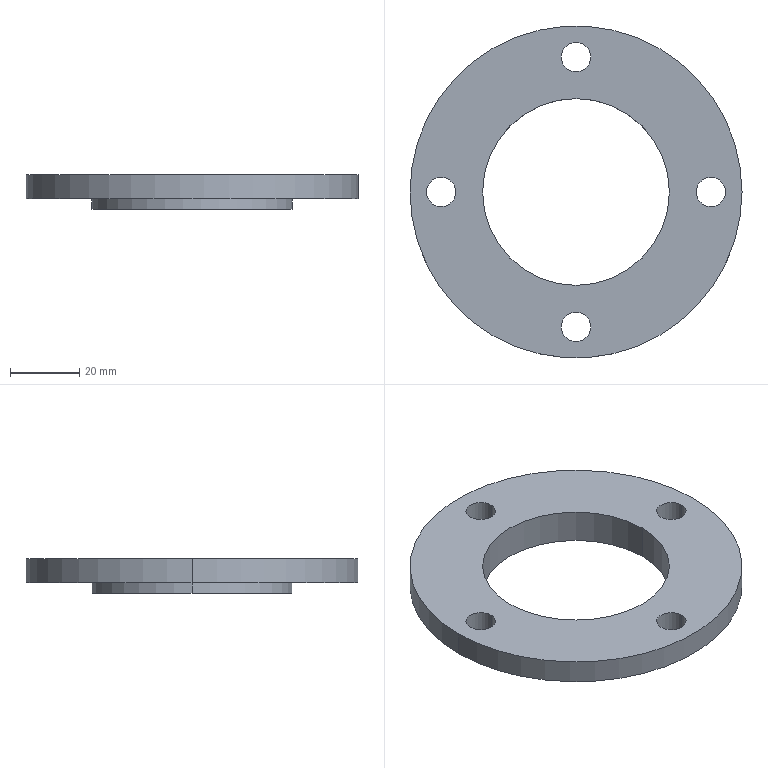Part | SolidWorks | features BaseBody 1 | 1 solid | 17 faces | box 96 x 96 x 10 mm | volume 34103 mm3 | cylinder 14 | plane 3 | commonest cylinder face diameters 8.5 x8 54 x2 58 x2 96 x2
STEP:
#1=CARTESIAN_POINT('',(29.,0.,-7.));
#2=VERTEX_POINT('',#1);
#3=CARTESIAN_POINT('',(29.,0.,-10.));
#4=VERTEX_POINT('',#3);
#5=CARTESIAN_POINT('',(29.,0.,-7.));
#6=DIRECTION('',(0.,0.,-1.));
#7=VECTOR('',#6,1000.);
#8=LINE('',#5,#7);
#9=EDGE_CURVE('',#2,#4,#8,.T.);
#10=ORIENTED_EDGE('',*,*,#9,.F.);
#11=CARTESIAN_POINT('',(-29.,0.,-7.));
#12=VERTEX_POINT('',#11);
#13=CARTESIAN_POINT('',(0.,0.,-7.));
#14=DIRECTION('',(0.,0.,-1.));
#15=DIRECTION('',(-1.,0.,0.));
#16=AXIS2_PLACEMENT_3D('',#13,#14,#15);
#17=CIRCLE('',#16,29.);
#18=EDGE_CURVE('',#2,#12,#17,.T.);
#19=ORIENTED_EDGE('',*,*,#18,.T.);
#20=CARTESIAN_POINT('',(-29.,0.,-10.));
#21=VERTEX_POINT('',#20);
#22=CARTESIAN_POINT('',(-29.,0.,-7.));
#23=DIRECTION('',(0.,0.,-1.));
#24=VECTOR('',#23,1000.);
#25=LINE('',#22,#24);
#26=EDGE_CURVE('',#12,#21,#25,.T.);
#27=ORIENTED_EDGE('',*,*,#26,.T.);
#28=CARTESIAN_POINT('',(0.,0.,-10.));
#29=DIRECTION('',(0.,0.,-1.));
#30=DIRECTION('',(-1.,0.,0.));
#31=AXIS2_PLACEMENT_3D('',#28,#29,#30);
#32=CIRCLE('',#31,29.);
#33=EDGE_CURVE('',#4,#21,#32,.T.);
#34=ORIENTED_EDGE('',*,*,#33,.F.);
#35=EDGE_LOOP('',(#10,#19,#27,#34));
#36=FACE_OUTER_BOUND('',#35,.T.);
#37=CARTESIAN_POINT('',(0.,0.,-7.));
#38=DIRECTION('',(0.,0.,-1.));
#39=DIRECTION('',(-1.,0.,0.));
#40=AXIS2_PLACEMENT_3D('',#37,#38,#39);
#41=CYLINDRICAL_SURFACE('',#40,29.);
#42=ADVANCED_FACE('',(#36),#41,.T.);
#43=CARTESIAN_POINT('',(4.25,39.,-7.));
#44=VERTEX_POINT('',#43);
#45=CARTESIAN_POINT('',(-4.25,39.,-7.));
#46=VERTEX_POINT('',#45);
#47=CARTESIAN_POINT('',(0.,39.,-7.));
#48=DIRECTION('',(0.,0.,1.));
#49=DIRECTION('',(-1.,0.,0.));
#50=AXIS2_PLACEMENT_3D('',#47,#48,#49);
#51=CIRCLE('',#50,4.25);
#52=EDGE_CURVE('',#44,#46,#51,.T.);
#53=ORIENTED_EDGE('',*,*,#52,.T.);
#54=CARTESIAN_POINT('',(0.,39.,-7.));
#55=DIRECTION('',(0.,0.,1.));
#56=DIRECTION('',(-1.,0.,0.));
#57=AXIS2_PLACEMENT_3D('',#54,#55,#56);
#58=CIRCLE('',#57,4.25);
#59=EDGE_CURVE('',#46,#44,#58,.T.);
#60=ORIENTED_EDGE('',*,*,#59,.T.);
#61=EDGE_LOOP('',(#53,#60));
#62=FACE_BOUND('',#61,.T.);
#63=CARTESIAN_POINT('',(43.25,0.,-7.));
#64=VERTEX_POINT('',#63);
#65=CARTESIAN_POINT('',(34.75,0.,-7.));
#66=VERTEX_POINT('',#65);
#67=CARTESIAN_POINT('',(39.,0.,-7.));
#68=DIRECTION('',(0.,0.,1.));
#69=DIRECTION('',(-1.,0.,0.));
#70=AXIS2_PLACEMENT_3D('',#67,#68,#69);
#71=CIRCLE('',#70,4.25);
#72=EDGE_CURVE('',#64,#66,#71,.T.);
#73=ORIENTED_EDGE('',*,*,#72,.T.);
#74=CARTESIAN_POINT('',(39.,0.,-7.));
#75=DIRECTION('',(0.,0.,1.));
#76=DIRECTION('',(-1.,0.,0.));
#77=AXIS2_PLACEMENT_3D('',#74,#75,#76);
#78=CIRCLE('',#77,4.25);
#79=EDGE_CURVE('',#66,#64,#78,.T.);
#80=ORIENTED_EDGE('',*,*,#79,.T.);
#81=EDGE_LOOP('',(#73,#80));
#82=FACE_BOUND('',#81,.T.);
#83=CARTESIAN_POINT('',(4.25,-39.,-7.));
#84=VERTEX_POINT('',#83);
#85=CARTESIAN_POINT('',(-4.25,-39.,-7.));
#86=VERTEX_POINT('',#85);
#87=CARTESIAN_POINT('',(0.,-39.,-7.));
#88=DIRECTION('',(0.,0.,1.));
#89=DIRECTION('',(-1.,0.,0.));
#90=AXIS2_PLACEMENT_3D('',#87,#88,#89);
#91=CIRCLE('',#90,4.25);
#92=EDGE_CURVE('',#84,#86,#91,.T.);
#93=ORIENTED_EDGE('',*,*,#92,.T.);
#94=CARTESIAN_POINT('',(0.,-39.,-7.));
#95=DIRECTION('',(0.,0.,1.));
#96=DIRECTION('',(-1.,0.,0.));
#97=AXIS2_PLACEMENT_3D('',#94,#95,#96);
#98=CIRCLE('',#97,4.25);
#99=EDGE_CURVE('',#86,#84,#98,.T.);
#100=ORIENTED_EDGE('',*,*,#99,.T.);
#101=EDGE_LOOP('',(#93,#100));
#102=FACE_BOUND('',#101,.T.);
#103=CARTESIAN_POINT('',(-34.75,0.,-7.));
#104=VERTEX_POINT('',#103);
#105=CARTESIAN_POINT('',(-43.25,0.,-7.));
#106=VERTEX_POINT('',#105);
#107=CARTESIAN_POINT('',(-39.,0.,-7.));
#108=DIRECTION('',(0.,0.,1.));
#109=DIRECTION('',(-1.,0.,0.));
#110=AXIS2_PLACEMENT_3D('',#107,#108,#109);
#111=CIRCLE('',#110,4.25);
#112=EDGE_CURVE('',#104,#106,#111,.T.);
#113=ORIENTED_EDGE('',*,*,#112,.T.);
#114=CARTESIAN_POINT('',(-39.,0.,-7.));
#115=DIRECTION('',(0.,0.,1.));
#116=DIRECTION('',(-1.,0.,0.));
#117=AXIS2_PLACEMENT_3D('',#114,#115,#116);
#118=CIRCLE('',#117,4.25);
#119=EDGE_CURVE('',#106,#104,#118,.T.);
#120=ORIENTED_EDGE('',*,*,#119,.T.);
#121=EDGE_LOOP('',(#113,#120));
#122=FACE_BOUND('',#121,.T.);
#123=CARTESIAN_POINT('',(0.,0.,-7.));
#124=DIRECTION('',(0.,0.,-1.));
#125=DIRECTION('',(-1.,0.,0.));
#126=AXIS2_PLACEMENT_3D('',#123,#124,#125);
#127=CIRCLE('',#126,29.);
#128=EDGE_CURVE('',#12,#2,#127,.T.);
#129=ORIENTED_EDGE('',*,*,#128,.F.);
#130=ORIENTED_EDGE('',*,*,#18,.F.);
#131=EDGE_LOOP('',(#129,#130));
#132=FACE_BOUND('',#131,.T.);
#133=CARTESIAN_POINT('',(48.,0.,-7.));
#134=VERTEX_POINT('',#133);
#135=CARTESIAN_POINT('',(-48.,0.,-7.));
#136=VERTEX_POINT('',#135);
#137=CARTESIAN_POINT('',(0.,0.,-7.));
#138=DIRECTION('',(0.,0.,1.));
#139=DIRECTION('',(-1.,0.,0.));
#140=AXIS2_PLACEMENT_3D('',#137,#138,#139);
#141=CIRCLE('',#140,48.);
#142=EDGE_CURVE('',#134,#136,#141,.T.);
#143=ORIENTED_EDGE('',*,*,#142,.F.);
#144=CARTESIAN_POINT('',(0.,0.,-7.));
#145=DIRECTION('',(0.,0.,1.));
#146=DIRECTION('',(-1.,0.,0.));
#147=AXIS2_PLACEMENT_3D('',#144,#145,#146);
#148=CIRCLE('',#147,48.);
#149=EDGE_CURVE('',#136,#134,#148,.T.);
#150=ORIENTED_EDGE('',*,*,#149,.F.);
#151=EDGE_LOOP('',(#143,#150));
#152=FACE_OUTER_BOUND('',#151,.T.);
#153=CARTESIAN_POINT('',(0.,0.,-7.));
#154=DIRECTION('',(0.,0.,-1.));
#155=DIRECTION('',(0.,-1.,0.));
#156=AXIS2_PLACEMENT_3D('',#153,#154,#155);
#157=PLANE('',#156);
#158=ADVANCED_FACE('',(#62,#82,#102,#122,#132,#152),#157,.T.);
#159=CARTESIAN_POINT('',(-27.,0.,-10.));
#160=VERTEX_POINT('',#159);
#161=CARTESIAN_POINT('',(-27.,0.,0.));
#162=VERTEX_POINT('',#161);
#163=CARTESIAN_POINT('',(-27.,0.,-10.));
#164=DIRECTION('',(0.,0.,1.));
#165=VECTOR('',#164,1000.);
#166=LINE('',#163,#165);
#167=EDGE_CURVE('',#160,#162,#166,.T.);
#168=ORIENTED_EDGE('',*,*,#167,.F.);
#169=CARTESIAN_POINT('',(27.,0.,-10.));
#170=VERTEX_POINT('',#169);
#171=CARTESIAN_POINT('',(0.,0.,-10.));
#172=DIRECTION('',(0.,0.,1.));
#173=DIRECTION('',(1.,0.,0.));
#174=AXIS2_PLACEMENT_3D('',#171,#172,#173);
#175=CIRCLE('',#174,27.);
#176=EDGE_CURVE('',#170,#160,#175,.T.);
#177=ORIENTED_EDGE('',*,*,#176,.F.);
#178=CARTESIAN_POINT('',(27.,0.,0.));
#179=VERTEX_POINT('',#178);
#180=CARTESIAN_POINT('',(27.,0.,-10.));
#181=DIRECTION('',(0.,0.,1.));
#182=VECTOR('',#181,1000.);
#183=LINE('',#180,#182);
#184=EDGE_CURVE('',#170,#179,#183,.T.);
#185=ORIENTED_EDGE('',*,*,#184,.T.);
#186=CARTESIAN_POINT('',(0.,0.,0.));
#187=DIRECTION('',(0.,0.,1.));
#188=DIRECTION('',(1.,0.,0.));
#189=AXIS2_PLACEMENT_3D('',#186,#187,#188);
#190=CIRCLE('',#189,27.);
#191=EDGE_CURVE('',#179,#162,#190,.T.);
#192=ORIENTED_EDGE('',*,*,#191,.T.);
#193=EDGE_LOOP('',(#168,#177,#185,#192));
#194=FACE_OUTER_BOUND('',#193,.T.);
#195=CARTESIAN_POINT('',(0.,0.,-10.));
#196=DIRECTION('',(0.,0.,1.));
#197=DIRECTION('',(1.,0.,0.));
#198=AXIS2_PLACEMENT_3D('',#195,#196,#197);
#199=CYLINDRICAL_SURFACE('',#198,27.);
#200=ADVANCED_FACE('',(#194),#199,.F.);
#201=ORIENTED_EDGE('',*,*,#191,.F.);
#202=CARTESIAN_POINT('',(0.,0.,0.));
#203=DIRECTION('',(0.,0.,1.));
#204=DIRECTION('',(1.,0.,0.));
#205=AXIS2_PLACEMENT_3D('',#202,#203,#204);
#206=CIRCLE('',#205,27.);
#207=EDGE_CURVE('',#162,#179,#206,.T.);
#208=ORIENTED_EDGE('',*,*,#207,.F.);
#209=EDGE_LOOP('',(#201,#208));
#210=FACE_BOUND('',#209,.T.);
#211=CARTESIAN_POINT('',(4.25,39.,0.));
#212=VERTEX_POINT('',#211);
#213=CARTESIAN_POINT('',(-4.25,39.,0.));
#214=VERTEX_POINT('',#213);
#215=CARTESIAN_POINT('',(0.,39.,0.));
#216=DIRECTION('',(0.,0.,1.));
#217=DIRECTION('',(1.,0.,0.));
#218=AXIS2_PLACEMENT_3D('',#215,#216,#217);
#219=CIRCLE('',#218,4.25);
#220=EDGE_CURVE('',#212,#214,#219,.T.);
#221=ORIENTED_EDGE('',*,*,#220,.F.);
#222=CARTESIAN_POINT('',(0.,39.,0.));
#223=DIRECTION('',(0.,0.,1.));
#224=DIRECTION('',(1.,0.,0.));
#225=AXIS2_PLACEMENT_3D('',#222,#223,#224);
#226=CIRCLE('',#225,4.25);
#227=EDGE_CURVE('',#214,#212,#226,.T.);
#228=ORIENTED_EDGE('',*,*,#227,.F.);
#229=EDGE_LOOP('',(#221,#228));
#230=FACE_BOUND('',#229,.T.);
#231=CARTESIAN_POINT('',(43.25,0.,0.));
#232=VERTEX_POINT('',#231);
#233=CARTESIAN_POINT('',(34.75,0.,0.));
#234=VERTEX_POINT('',#233);
#235=CARTESIAN_POINT('',(39.,0.,0.));
#236=DIRECTION('',(0.,0.,1.));
#237=DIRECTION('',(0.,-1.,0.));
#238=AXIS2_PLACEMENT_3D('',#235,#236,#237);
#239=CIRCLE('',#238,4.25);
#240=EDGE_CURVE('',#232,#234,#239,.T.);
#241=ORIENTED_EDGE('',*,*,#240,.F.);
#242=CARTESIAN_POINT('',(39.,0.,0.));
#243=DIRECTION('',(0.,0.,1.));
#244=DIRECTION('',(0.,-1.,0.));
#245=AXIS2_PLACEMENT_3D('',#242,#243,#244);
#246=CIRCLE('',#245,4.25);
#247=EDGE_CURVE('',#234,#232,#246,.T.);
#248=ORIENTED_EDGE('',*,*,#247,.F.);
#249=EDGE_LOOP('',(#241,#248));
#250=FACE_BOUND('',#249,.T.);
#251=CARTESIAN_POINT('',(4.25,-39.,0.));
#252=VERTEX_POINT('',#251);
#253=CARTESIAN_POINT('',(-4.25,-39.,0.));
#254=VERTEX_POINT('',#253);
#255=CARTESIAN_POINT('',(0.,-39.,0.));
#256=DIRECTION('',(0.,0.,1.));
#257=DIRECTION('',(-1.,0.,0.));
#258=AXIS2_PLACEMENT_3D('',#255,#256,#257);
#259=CIRCLE('',#258,4.25);
#260=EDGE_CURVE('',#252,#254,#259,.T.);
#261=ORIENTED_EDGE('',*,*,#260,.F.);
#262=CARTESIAN_POINT('',(0.,-39.,0.));
#263=DIRECTION('',(0.,0.,1.));
#264=DIRECTION('',(-1.,0.,0.));
#265=AXIS2_PLACEMENT_3D('',#262,#263,#264);
#266=CIRCLE('',#265,4.25);
#267=EDGE_CURVE('',#254,#252,#266,.T.);
#268=ORIENTED_EDGE('',*,*,#267,.F.);
#269=EDGE_LOOP('',(#261,#268));
#270=FACE_BOUND('',#269,.T.);
#271=CARTESIAN_POINT('',(-34.75,0.,0.));
#272=VERTEX_POINT('',#271);
#273=CARTESIAN_POINT('',(-43.25,0.,0.));
#274=VERTEX_POINT('',#273);
#275=CARTESIAN_POINT('',(-39.,0.,0.));
#276=DIRECTION('',(0.,0.,1.));
#277=DIRECTION('',(0.,1.,0.));
#278=AXIS2_PLACEMENT_3D('',#275,#276,#277);
#279=CIRCLE('',#278,4.25);
#280=EDGE_CURVE('',#272,#274,#279,.T.);
#281=ORIENTED_EDGE('',*,*,#280,.F.);
#282=CARTESIAN_POINT('',(-39.,0.,0.));
#283=DIRECTION('',(0.,0.,1.));
#284=DIRECTION('',(0.,1.,0.));
#285=AXIS2_PLACEMENT_3D('',#282,#283,#284);
#286=CIRCLE('',#285,4.25);
#287=EDGE_CURVE('',#274,#272,#286,.T.);
#288=ORIENTED_EDGE('',*,*,#287,.F.);
#289=EDGE_LOOP('',(#281,#288));
#290=FACE_BOUND('',#289,.T.);
#291=CARTESIAN_POINT('',(48.,0.,0.));
#292=VERTEX_POINT('',#291);
#293=CARTESIAN_POINT('',(-48.,0.,0.));
#294=VERTEX_POINT('',#293);
#295=CARTESIAN_POINT('',(0.,0.,0.));
#296=DIRECTION('',(0.,0.,1.));
#297=DIRECTION('',(1.,0.,0.));
#298=AXIS2_PLACEMENT_3D('',#295,#296,#297);
#299=CIRCLE('',#298,48.);
#300=EDGE_CURVE('',#292,#294,#299,.T.);
#301=ORIENTED_EDGE('',*,*,#300,.T.);
#302=CARTESIAN_POINT('',(0.,0.,0.));
#303=DIRECTION('',(0.,0.,1.));
#304=DIRECTION('',(1.,0.,0.));
#305=AXIS2_PLACEMENT_3D('',#302,#303,#304);
#306=CIRCLE('',#305,48.);
#307=EDGE_CURVE('',#294,#292,#306,.T.);
#308=ORIENTED_EDGE('',*,*,#307,.T.);
#309=EDGE_LOOP('',(#301,#308));
#310=FACE_OUTER_BOUND('',#309,.T.);
#311=CARTESIAN_POINT('',(0.,0.,0.));
#312=DIRECTION('',(0.,0.,1.));
#313=DIRECTION('',(1.,0.,0.));
#314=AXIS2_PLACEMENT_3D('',#311,#312,#313);
#315=PLANE('',#314);
#316=ADVANCED_FACE('',(#210,#230,#250,#270,#290,#310),#315,.T.);
#317=CARTESIAN_POINT('',(-43.25,0.,-10.));
#318=DIRECTION('',(0.,0.,1.));
#319=VECTOR('',#318,1000.);
#320=LINE('',#317,#319);
#321=EDGE_CURVE('',#106,#274,#320,.T.);
#322=ORIENTED_EDGE('',*,*,#321,.F.);
#323=ORIENTED_EDGE('',*,*,#112,.F.);
#324=CARTESIAN_POINT('',(-34.75,0.,-10.));
#325=DIRECTION('',(0.,0.,1.));
#326=VECTOR('',#325,1000.);
#327=LINE('',#324,#326);
#328=EDGE_CURVE('',#104,#272,#327,.T.);
#329=ORIENTED_EDGE('',*,*,#328,.T.);
#330=ORIENTED_EDGE('',*,*,#280,.T.);
#331=EDGE_LOOP('',(#322,#323,#329,#330));
#332=FACE_OUTER_BOUND('',#331,.T.);
#333=CARTESIAN_POINT('',(-39.,0.,-10.));
#334=DIRECTION('',(0.,0.,1.));
#335=DIRECTION('',(1.,0.,0.));
#336=AXIS2_PLACEMENT_3D('',#333,#334,#335);
#337=CYLINDRICAL_SURFACE('',#336,4.25);
#338=ADVANCED_FACE('',(#332),#337,.F.);
#339=CARTESIAN_POINT('',(-4.25,-39.,-10.));
#340=DIRECTION('',(0.,0.,1.));
#341=VECTOR('',#340,1000.);
#342=LINE('',#339,#341);
#343=EDGE_CURVE('',#86,#254,#342,.T.);
#344=ORIENTED_EDGE('',*,*,#343,.F.);
#345=ORIENTED_EDGE('',*,*,#92,.F.);
#346=CARTESIAN_POINT('',(4.25,-39.,-10.));
#347=DIRECTION('',(0.,0.,1.));
#348=VECTOR('',#347,1000.);
#349=LINE('',#346,#348);
#350=EDGE_CURVE('',#84,#252,#349,.T.);
#351=ORIENTED_EDGE('',*,*,#350,.T.);
#352=ORIENTED_EDGE('',*,*,#260,.T.);
#353=EDGE_LOOP('',(#344,#345,#351,#352));
#354=FACE_OUTER_BOUND('',#353,.T.);
#355=CARTESIAN_POINT('',(0.,-39.,-10.));
#356=DIRECTION('',(0.,0.,1.));
#357=DIRECTION('',(1.,0.,0.));
#358=AXIS2_PLACEMENT_3D('',#355,#356,#357);
#359=CYLINDRICAL_SURFACE('',#358,4.25);
#360=ADVANCED_FACE('',(#354),#359,.F.);
#361=CARTESIAN_POINT('',(34.75,0.,-10.));
#362=DIRECTION('',(0.,0.,1.));
#363=VECTOR('',#362,1000.);
#364=LINE('',#361,#363);
#365=EDGE_CURVE('',#66,#234,#364,.T.);
#366=ORIENTED_EDGE('',*,*,#365,.F.);
#367=ORIENTED_EDGE('',*,*,#72,.F.);
#368=CARTESIAN_POINT('',(43.25,0.,-10.));
#369=DIRECTION('',(0.,0.,1.));
#370=VECTOR('',#369,1000.);
#371=LINE('',#368,#370);
#372=EDGE_CURVE('',#64,#232,#371,.T.);
#373=ORIENTED_EDGE('',*,*,#372,.T.);
#374=ORIENTED_EDGE('',*,*,#240,.T.);
#375=EDGE_LOOP('',(#366,#367,#373,#374));
#376=FACE_OUTER_BOUND('',#375,.T.);
#377=CARTESIAN_POINT('',(39.,0.,-10.));
#378=DIRECTION('',(0.,0.,1.));
#379=DIRECTION('',(1.,0.,0.));
#380=AXIS2_PLACEMENT_3D('',#377,#378,#379);
#381=CYLINDRICAL_SURFACE('',#380,4.25);
#382=ADVANCED_FACE('',(#376),#381,.F.);
#383=CARTESIAN_POINT('',(-4.25,39.,-10.));
#384=DIRECTION('',(0.,0.,1.));
#385=VECTOR('',#384,1000.);
#386=LINE('',#383,#385);
#387=EDGE_CURVE('',#46,#214,#386,.T.);
#388=ORIENTED_EDGE('',*,*,#387,.F.);
#389=ORIENTED_EDGE('',*,*,#52,.F.);
#390=CARTESIAN_POINT('',(4.25,39.,-10.));
#391=DIRECTION('',(0.,0.,1.));
#392=VECTOR('',#391,1000.);
#393=LINE('',#390,#392);
#394=EDGE_CURVE('',#44,#212,#393,.T.);
#395=ORIENTED_EDGE('',*,*,#394,.T.);
#396=ORIENTED_EDGE('',*,*,#220,.T.);
#397=EDGE_LOOP('',(#388,#389,#395,#396));
#398=FACE_OUTER_BOUND('',#397,.T.);
#399=CARTESIAN_POINT('',(0.,39.,-10.));
#400=DIRECTION('',(0.,0.,1.));
#401=DIRECTION('',(1.,0.,0.));
#402=AXIS2_PLACEMENT_3D('',#399,#400,#401);
#403=CYLINDRICAL_SURFACE('',#402,4.25);
#404=ADVANCED_FACE('',(#398),#403,.F.);
#405=ORIENTED_EDGE('',*,*,#176,.T.);
#406=CARTESIAN_POINT('',(0.,0.,-10.));
#407=DIRECTION('',(0.,0.,1.));
#408=DIRECTION('',(1.,0.,0.));
#409=AXIS2_PLACEMENT_3D('',#406,#407,#408);
#410=CIRCLE('',#409,27.);
#411=EDGE_CURVE('',#160,#170,#410,.T.);
#412=ORIENTED_EDGE('',*,*,#411,.T.);
#413=EDGE_LOOP('',(#405,#412));
#414=FACE_BOUND('',#413,.T.);
#415=CARTESIAN_POINT('',(0.,0.,-10.));
#416=DIRECTION('',(0.,0.,-1.));
#417=DIRECTION('',(-1.,0.,0.));
#418=AXIS2_PLACEMENT_3D('',#415,#416,#417);
#419=CIRCLE('',#418,29.);
#420=EDGE_CURVE('',#21,#4,#419,.T.);
#421=ORIENTED_EDGE('',*,*,#420,.T.);
#422=ORIENTED_EDGE('',*,*,#33,.T.);
#423=EDGE_LOOP('',(#421,#422));
#424=FACE_OUTER_BOUND('',#423,.T.);
#425=CARTESIAN_POINT('',(0.,0.,-10.));
#426=DIRECTION('',(0.,0.,1.));
#427=DIRECTION('',(1.,0.,0.));
#428=AXIS2_PLACEMENT_3D('',#425,#426,#427);
#429=PLANE('',#428);
#430=ADVANCED_FACE('',(#414,#424),#429,.F.);
#431=CARTESIAN_POINT('',(-48.,0.,-10.));
#432=DIRECTION('',(0.,0.,1.));
#433=VECTOR('',#432,1000.);
#434=LINE('',#431,#433);
#435=EDGE_CURVE('',#136,#294,#434,.T.);
#436=ORIENTED_EDGE('',*,*,#435,.F.);
#437=ORIENTED_EDGE('',*,*,#149,.T.);
#438=CARTESIAN_POINT('',(48.,0.,-10.));
#439=DIRECTION('',(0.,0.,1.));
#440=VECTOR('',#439,1000.);
#441=LINE('',#438,#440);
#442=EDGE_CURVE('',#134,#292,#441,.T.);
#443=ORIENTED_EDGE('',*,*,#442,.T.);
#444=ORIENTED_EDGE('',*,*,#307,.F.);
#445=EDGE_LOOP('',(#436,#437,#443,#444));
#446=FACE_OUTER_BOUND('',#445,.T.);
#447=CARTESIAN_POINT('',(0.,0.,-10.));
#448=DIRECTION('',(0.,0.,1.));
#449=DIRECTION('',(1.,0.,0.));
#450=AXIS2_PLACEMENT_3D('',#447,#448,#449);
#451=CYLINDRICAL_SURFACE('',#450,48.);
#452=ADVANCED_FACE('',(#446),#451,.T.);
#453=ORIENTED_EDGE('',*,*,#142,.T.);
#454=ORIENTED_EDGE('',*,*,#435,.T.);
#455=ORIENTED_EDGE('',*,*,#300,.F.);
#456=ORIENTED_EDGE('',*,*,#442,.F.);
#457=EDGE_LOOP('',(#453,#454,#455,#456));
#458=FACE_OUTER_BOUND('',#457,.T.);
#459=CARTESIAN_POINT('',(0.,0.,-10.));
#460=DIRECTION('',(0.,0.,1.));
#461=DIRECTION('',(1.,0.,0.));
#462=AXIS2_PLACEMENT_3D('',#459,#460,#461);
#463=CYLINDRICAL_SURFACE('',#462,48.);
#464=ADVANCED_FACE('',(#458),#463,.T.);
#465=ORIENTED_EDGE('',*,*,#59,.F.);
#466=ORIENTED_EDGE('',*,*,#387,.T.);
#467=ORIENTED_EDGE('',*,*,#227,.T.);
#468=ORIENTED_EDGE('',*,*,#394,.F.);
#469=EDGE_LOOP('',(#465,#466,#467,#468));
#470=FACE_OUTER_BOUND('',#469,.T.);
#471=CARTESIAN_POINT('',(0.,39.,-10.));
#472=DIRECTION('',(0.,0.,1.));
#473=DIRECTION('',(1.,0.,0.));
#474=AXIS2_PLACEMENT_3D('',#471,#472,#473);
#475=CYLINDRICAL_SURFACE('',#474,4.25);
#476=ADVANCED_FACE('',(#470),#475,.F.);
#477=ORIENTED_EDGE('',*,*,#79,.F.);
#478=ORIENTED_EDGE('',*,*,#365,.T.);
#479=ORIENTED_EDGE('',*,*,#247,.T.);
#480=ORIENTED_EDGE('',*,*,#372,.F.);
#481=EDGE_LOOP('',(#477,#478,#479,#480));
#482=FACE_OUTER_BOUND('',#481,.T.);
#483=CARTESIAN_POINT('',(39.,0.,-10.));
#484=DIRECTION('',(0.,0.,1.));
#485=DIRECTION('',(1.,0.,0.));
#486=AXIS2_PLACEMENT_3D('',#483,#484,#485);
#487=CYLINDRICAL_SURFACE('',#486,4.25);
#488=ADVANCED_FACE('',(#482),#487,.F.);
#489=ORIENTED_EDGE('',*,*,#99,.F.);
#490=ORIENTED_EDGE('',*,*,#343,.T.);
#491=ORIENTED_EDGE('',*,*,#267,.T.);
#492=ORIENTED_EDGE('',*,*,#350,.F.);
#493=EDGE_LOOP('',(#489,#490,#491,#492));
#494=FACE_OUTER_BOUND('',#493,.T.);
#495=CARTESIAN_POINT('',(0.,-39.,-10.));
#496=DIRECTION('',(0.,0.,1.));
#497=DIRECTION('',(1.,0.,0.));
#498=AXIS2_PLACEMENT_3D('',#495,#496,#497);
#499=CYLINDRICAL_SURFACE('',#498,4.25);
#500=ADVANCED_FACE('',(#494),#499,.F.);
#501=ORIENTED_EDGE('',*,*,#119,.F.);
#502=ORIENTED_EDGE('',*,*,#321,.T.);
#503=ORIENTED_EDGE('',*,*,#287,.T.);
#504=ORIENTED_EDGE('',*,*,#328,.F.);
#505=EDGE_LOOP('',(#501,#502,#503,#504));
#506=FACE_OUTER_BOUND('',#505,.T.);
#507=CARTESIAN_POINT('',(-39.,0.,-10.));
#508=DIRECTION('',(0.,0.,1.));
#509=DIRECTION('',(1.,0.,0.));
#510=AXIS2_PLACEMENT_3D('',#507,#508,#509);
#511=CYLINDRICAL_SURFACE('',#510,4.25);
#512=ADVANCED_FACE('',(#506),#511,.F.);
#513=ORIENTED_EDGE('',*,*,#411,.F.);
#514=ORIENTED_EDGE('',*,*,#167,.T.);
#515=ORIENTED_EDGE('',*,*,#207,.T.);
#516=ORIENTED_EDGE('',*,*,#184,.F.);
#517=EDGE_LOOP('',(#513,#514,#515,#516));
#518=FACE_OUTER_BOUND('',#517,.T.);
#519=CARTESIAN_POINT('',(0.,0.,-10.));
#520=DIRECTION('',(0.,0.,1.));
#521=DIRECTION('',(1.,0.,0.));
#522=AXIS2_PLACEMENT_3D('',#519,#520,#521);
#523=CYLINDRICAL_SURFACE('',#522,27.);
#524=ADVANCED_FACE('',(#518),#523,.F.);
#525=ORIENTED_EDGE('',*,*,#128,.T.);
#526=ORIENTED_EDGE('',*,*,#9,.T.);
#527=ORIENTED_EDGE('',*,*,#420,.F.);
#528=ORIENTED_EDGE('',*,*,#26,.F.);
#529=EDGE_LOOP('',(#525,#526,#527,#528));
#530=FACE_OUTER_BOUND('',#529,.T.);
#531=CARTESIAN_POINT('',(0.,0.,-7.));
#532=DIRECTION('',(0.,0.,-1.));
#533=DIRECTION('',(-1.,0.,0.));
#534=AXIS2_PLACEMENT_3D('',#531,#532,#533);
#535=CYLINDRICAL_SURFACE('',#534,29.);
#536=ADVANCED_FACE('',(#530),#535,.T.);
#537=CLOSED_SHELL('',(#42,#158,#200,#316,#338,#360,#382,#404,#430,#452,#464,#476,#488,#500,#512,#524,#536));
#538=MANIFOLD_SOLID_BREP('',#537);
#539=CARTESIAN_POINT('',(0.,0.,0.));
#540=DIRECTION('',(0.,0.,1.));
#541=DIRECTION('',(1.,0.,0.));
#542=AXIS2_PLACEMENT_3D('',#539,#540,#541);
#543=(LENGTH_UNIT()NAMED_UNIT(*)SI_UNIT(.MILLI.,.METRE.));
#544=UNCERTAINTY_MEASURE_WITH_UNIT(LENGTH_MEASURE(0.00001),#543,'','');
#545=(NAMED_UNIT(*)PLANE_ANGLE_UNIT()SI_UNIT($,.RADIAN.));
#546=(NAMED_UNIT(*)SI_UNIT($,.STERADIAN.)SOLID_ANGLE_UNIT());
#547=(GEOMETRIC_REPRESENTATION_CONTEXT(3)GLOBAL_UNCERTAINTY_ASSIGNED_CONTEXT((#544))GLOBAL_UNIT_ASSIGNED_CONTEXT((#543,#545,#546))REPRESENTATION_CONTEXT('',''));
#548=ADVANCED_BREP_SHAPE_REPRESENTATION('',(#538,#542),#547);